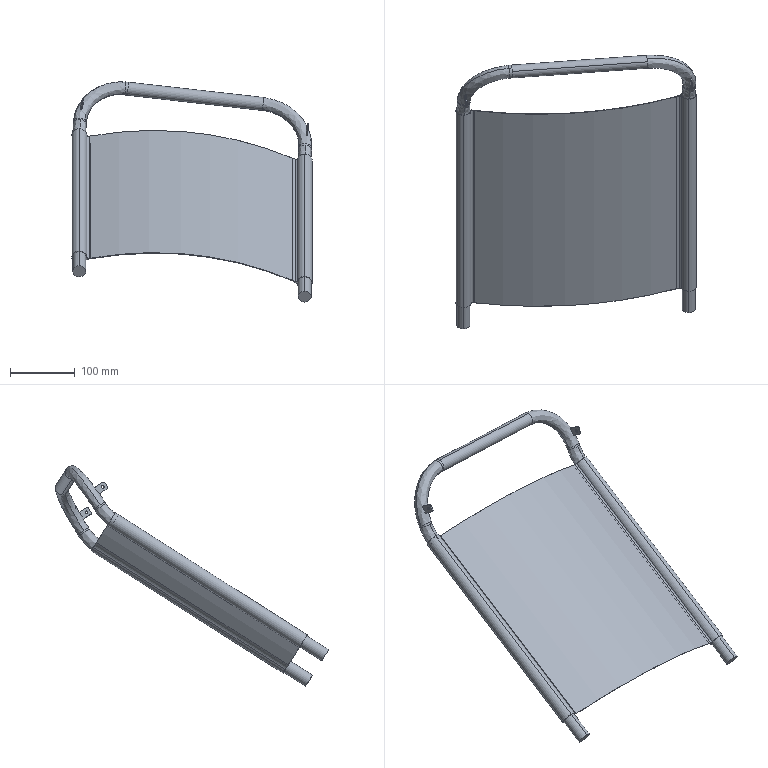Part | SolidWorks | features BaseBody 2 | 2 solids | 61 faces | box 369.895 x 420.824 x 339.005 mm | volume 568588 mm3 | cylinder 29 | plane 16 | spline 16 | commonest cylinder face diameters 20 x10 4 x5 4.2 x4 23 x3 23.373 x3 21 x2